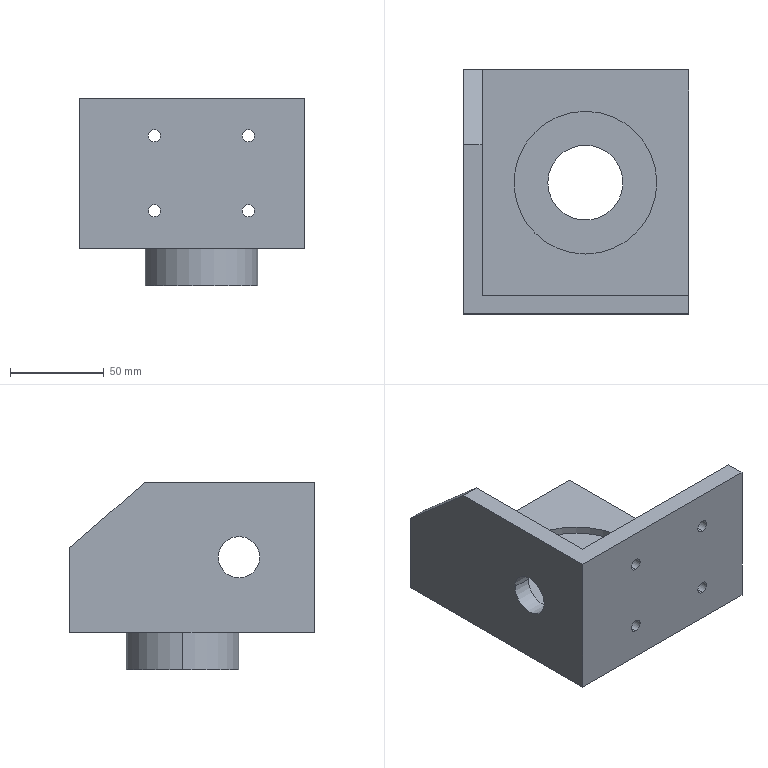Part | NX | features BREP 1 | 1 solid | 31 faces | box 120 x 130 x 100 mm | volume 300260 mm3 | cylinder 18 | plane 13 | commonest cylinder face diameters 6.5 x8 22 x2 40 x2 52 x2 60 x2 76 x2
STEP:
#1=CARTESIAN_POINT('',(-30.,0.,20.));
#2=VERTEX_POINT('',#1);
#3=CARTESIAN_POINT('',(30.,0.,20.));
#4=VERTEX_POINT('',#3);
#5=CARTESIAN_POINT('',(0.,0.,20.));
#6=DIRECTION('',(0.,0.,-1.));
#7=DIRECTION('',(-1.,0.,0.));
#8=AXIS2_PLACEMENT_3D('',#5,#6,#7);
#9=CIRCLE('',#8,30.);
#10=EDGE_CURVE('',#2,#4,#9,.T.);
#11=ORIENTED_EDGE('',*,*,#10,.T.);
#12=CARTESIAN_POINT('',(30.,0.,0.));
#13=VERTEX_POINT('',#12);
#14=CARTESIAN_POINT('',(30.,0.,20.));
#15=DIRECTION('',(0.,0.,-1.));
#16=VECTOR('',#15,1000.);
#17=LINE('',#14,#16);
#18=EDGE_CURVE('',#4,#13,#17,.T.);
#19=ORIENTED_EDGE('',*,*,#18,.T.);
#20=CARTESIAN_POINT('',(-30.,0.,0.));
#21=VERTEX_POINT('',#20);
#22=CARTESIAN_POINT('',(0.,0.,0.));
#23=DIRECTION('',(0.,0.,1.));
#24=DIRECTION('',(-1.,0.,0.));
#25=AXIS2_PLACEMENT_3D('',#22,#23,#24);
#26=CIRCLE('',#25,30.);
#27=EDGE_CURVE('',#13,#21,#26,.T.);
#28=ORIENTED_EDGE('',*,*,#27,.T.);
#29=CARTESIAN_POINT('',(-30.,0.,20.));
#30=DIRECTION('',(0.,0.,-1.));
#31=VECTOR('',#30,1000.);
#32=LINE('',#29,#31);
#33=EDGE_CURVE('',#2,#21,#32,.T.);
#34=ORIENTED_EDGE('',*,*,#33,.F.);
#35=EDGE_LOOP('',(#11,#19,#28,#34));
#36=FACE_BOUND('',#35,.T.);
#37=CARTESIAN_POINT('',(0.,0.,20.));
#38=DIRECTION('',(0.,0.,-1.));
#39=DIRECTION('',(-1.,0.,0.));
#40=AXIS2_PLACEMENT_3D('',#37,#38,#39);
#41=CYLINDRICAL_SURFACE('',#40,30.);
#42=ADVANCED_FACE('',(#36),#41,.T.);
#43=CARTESIAN_POINT('',(-25.,-60.,83.25));
#44=VERTEX_POINT('',#43);
#45=CARTESIAN_POINT('',(-25.,-60.,76.75));
#46=VERTEX_POINT('',#45);
#47=CARTESIAN_POINT('',(-25.,-60.,80.));
#48=DIRECTION('',(0.,-1.,0.));
#49=DIRECTION('',(0.,0.,-1.));
#50=AXIS2_PLACEMENT_3D('',#47,#48,#49);
#51=CIRCLE('',#50,3.25);
#52=EDGE_CURVE('',#44,#46,#51,.T.);
#53=ORIENTED_EDGE('',*,*,#52,.F.);
#54=CARTESIAN_POINT('',(-25.,-70.,83.25));
#55=VERTEX_POINT('',#54);
#56=CARTESIAN_POINT('',(-25.,-60.,83.25));
#57=DIRECTION('',(0.,-1.,0.));
#58=VECTOR('',#57,1000.);
#59=LINE('',#56,#58);
#60=EDGE_CURVE('',#44,#55,#59,.T.);
#61=ORIENTED_EDGE('',*,*,#60,.T.);
#62=CARTESIAN_POINT('',(-25.,-70.,76.75));
#63=VERTEX_POINT('',#62);
#64=CARTESIAN_POINT('',(-25.,-70.,80.));
#65=DIRECTION('',(0.,1.,0.));
#66=DIRECTION('',(0.,0.,-1.));
#67=AXIS2_PLACEMENT_3D('',#64,#65,#66);
#68=CIRCLE('',#67,3.25);
#69=EDGE_CURVE('',#63,#55,#68,.T.);
#70=ORIENTED_EDGE('',*,*,#69,.F.);
#71=CARTESIAN_POINT('',(-25.,-60.,76.75));
#72=DIRECTION('',(0.,-1.,0.));
#73=VECTOR('',#72,1000.);
#74=LINE('',#71,#73);
#75=EDGE_CURVE('',#46,#63,#74,.T.);
#76=ORIENTED_EDGE('',*,*,#75,.F.);
#77=EDGE_LOOP('',(#53,#61,#70,#76));
#78=FACE_BOUND('',#77,.T.);
#79=CARTESIAN_POINT('',(-25.,-60.,80.));
#80=DIRECTION('',(0.,-1.,0.));
#81=DIRECTION('',(0.,0.,-1.));
#82=AXIS2_PLACEMENT_3D('',#79,#80,#81);
#83=CYLINDRICAL_SURFACE('',#82,3.25);
#84=ADVANCED_FACE('',(#78),#83,.F.);
#85=CARTESIAN_POINT('',(25.,-60.,83.25));
#86=VERTEX_POINT('',#85);
#87=CARTESIAN_POINT('',(25.,-60.,76.75));
#88=VERTEX_POINT('',#87);
#89=CARTESIAN_POINT('',(25.,-60.,80.));
#90=DIRECTION('',(0.,-1.,0.));
#91=DIRECTION('',(0.,0.,-1.));
#92=AXIS2_PLACEMENT_3D('',#89,#90,#91);
#93=CIRCLE('',#92,3.25);
#94=EDGE_CURVE('',#86,#88,#93,.T.);
#95=ORIENTED_EDGE('',*,*,#94,.F.);
#96=CARTESIAN_POINT('',(25.,-70.,83.25));
#97=VERTEX_POINT('',#96);
#98=CARTESIAN_POINT('',(25.,-60.,83.25));
#99=DIRECTION('',(0.,-1.,0.));
#100=VECTOR('',#99,1000.);
#101=LINE('',#98,#100);
#102=EDGE_CURVE('',#86,#97,#101,.T.);
#103=ORIENTED_EDGE('',*,*,#102,.T.);
#104=CARTESIAN_POINT('',(25.,-70.,76.75));
#105=VERTEX_POINT('',#104);
#106=CARTESIAN_POINT('',(25.,-70.,80.));
#107=DIRECTION('',(0.,1.,0.));
#108=DIRECTION('',(0.,0.,-1.));
#109=AXIS2_PLACEMENT_3D('',#106,#107,#108);
#110=CIRCLE('',#109,3.25);
#111=EDGE_CURVE('',#105,#97,#110,.T.);
#112=ORIENTED_EDGE('',*,*,#111,.F.);
#113=CARTESIAN_POINT('',(25.,-60.,76.75));
#114=DIRECTION('',(0.,-1.,0.));
#115=VECTOR('',#114,1000.);
#116=LINE('',#113,#115);
#117=EDGE_CURVE('',#88,#105,#116,.T.);
#118=ORIENTED_EDGE('',*,*,#117,.F.);
#119=EDGE_LOOP('',(#95,#103,#112,#118));
#120=FACE_BOUND('',#119,.T.);
#121=CARTESIAN_POINT('',(25.,-60.,80.));
#122=DIRECTION('',(0.,-1.,0.));
#123=DIRECTION('',(0.,0.,-1.));
#124=AXIS2_PLACEMENT_3D('',#121,#122,#123);
#125=CYLINDRICAL_SURFACE('',#124,3.25);
#126=ADVANCED_FACE('',(#120),#125,.F.);
#127=CARTESIAN_POINT('',(25.,-60.,43.25));
#128=VERTEX_POINT('',#127);
#129=CARTESIAN_POINT('',(25.,-60.,36.75));
#130=VERTEX_POINT('',#129);
#131=CARTESIAN_POINT('',(25.,-60.,40.));
#132=DIRECTION('',(0.,-1.,0.));
#133=DIRECTION('',(0.,0.,-1.));
#134=AXIS2_PLACEMENT_3D('',#131,#132,#133);
#135=CIRCLE('',#134,3.25);
#136=EDGE_CURVE('',#128,#130,#135,.T.);
#137=ORIENTED_EDGE('',*,*,#136,.F.);
#138=CARTESIAN_POINT('',(25.,-70.,43.25));
#139=VERTEX_POINT('',#138);
#140=CARTESIAN_POINT('',(25.,-60.,43.25));
#141=DIRECTION('',(0.,-1.,0.));
#142=VECTOR('',#141,1000.);
#143=LINE('',#140,#142);
#144=EDGE_CURVE('',#128,#139,#143,.T.);
#145=ORIENTED_EDGE('',*,*,#144,.T.);
#146=CARTESIAN_POINT('',(25.,-70.,36.75));
#147=VERTEX_POINT('',#146);
#148=CARTESIAN_POINT('',(25.,-70.,40.));
#149=DIRECTION('',(0.,1.,0.));
#150=DIRECTION('',(0.,0.,-1.));
#151=AXIS2_PLACEMENT_3D('',#148,#149,#150);
#152=CIRCLE('',#151,3.25);
#153=EDGE_CURVE('',#147,#139,#152,.T.);
#154=ORIENTED_EDGE('',*,*,#153,.F.);
#155=CARTESIAN_POINT('',(25.,-60.,36.75));
#156=DIRECTION('',(0.,-1.,0.));
#157=VECTOR('',#156,1000.);
#158=LINE('',#155,#157);
#159=EDGE_CURVE('',#130,#147,#158,.T.);
#160=ORIENTED_EDGE('',*,*,#159,.F.);
#161=EDGE_LOOP('',(#137,#145,#154,#160));
#162=FACE_BOUND('',#161,.T.);
#163=CARTESIAN_POINT('',(25.,-60.,40.));
#164=DIRECTION('',(0.,-1.,0.));
#165=DIRECTION('',(0.,0.,-1.));
#166=AXIS2_PLACEMENT_3D('',#163,#164,#165);
#167=CYLINDRICAL_SURFACE('',#166,3.25);
#168=ADVANCED_FACE('',(#162),#167,.F.);
#169=CARTESIAN_POINT('',(-25.,-60.,43.25));
#170=VERTEX_POINT('',#169);
#171=CARTESIAN_POINT('',(-25.,-60.,36.75));
#172=VERTEX_POINT('',#171);
#173=CARTESIAN_POINT('',(-25.,-60.,40.));
#174=DIRECTION('',(0.,-1.,0.));
#175=DIRECTION('',(0.,0.,-1.));
#176=AXIS2_PLACEMENT_3D('',#173,#174,#175);
#177=CIRCLE('',#176,3.25);
#178=EDGE_CURVE('',#170,#172,#177,.T.);
#179=ORIENTED_EDGE('',*,*,#178,.F.);
#180=CARTESIAN_POINT('',(-25.,-70.,43.25));
#181=VERTEX_POINT('',#180);
#182=CARTESIAN_POINT('',(-25.,-60.,43.25));
#183=DIRECTION('',(0.,-1.,0.));
#184=VECTOR('',#183,1000.);
#185=LINE('',#182,#184);
#186=EDGE_CURVE('',#170,#181,#185,.T.);
#187=ORIENTED_EDGE('',*,*,#186,.T.);
#188=CARTESIAN_POINT('',(-25.,-70.,36.75));
#189=VERTEX_POINT('',#188);
#190=CARTESIAN_POINT('',(-25.,-70.,40.));
#191=DIRECTION('',(0.,1.,0.));
#192=DIRECTION('',(0.,0.,-1.));
#193=AXIS2_PLACEMENT_3D('',#190,#191,#192);
#194=CIRCLE('',#193,3.25);
#195=EDGE_CURVE('',#189,#181,#194,.T.);
#196=ORIENTED_EDGE('',*,*,#195,.F.);
#197=CARTESIAN_POINT('',(-25.,-60.,36.75));
#198=DIRECTION('',(0.,-1.,0.));
#199=VECTOR('',#198,1000.);
#200=LINE('',#197,#199);
#201=EDGE_CURVE('',#172,#189,#200,.T.);
#202=ORIENTED_EDGE('',*,*,#201,.F.);
#203=EDGE_LOOP('',(#179,#187,#196,#202));
#204=FACE_BOUND('',#203,.T.);
#205=CARTESIAN_POINT('',(-25.,-60.,40.));
#206=DIRECTION('',(0.,-1.,0.));
#207=DIRECTION('',(0.,0.,-1.));
#208=AXIS2_PLACEMENT_3D('',#205,#206,#207);
#209=CYLINDRICAL_SURFACE('',#208,3.25);
#210=ADVANCED_FACE('',(#204),#209,.F.);
#211=CARTESIAN_POINT('',(-55.,-19.,60.));
#212=VERTEX_POINT('',#211);
#213=CARTESIAN_POINT('',(-55.,-41.,60.));
#214=VERTEX_POINT('',#213);
#215=CARTESIAN_POINT('',(-55.,-30.,60.));
#216=DIRECTION('',(-1.,0.,0.));
#217=DIRECTION('',(0.,-1.,0.));
#218=AXIS2_PLACEMENT_3D('',#215,#216,#217);
#219=CIRCLE('',#218,11.);
#220=EDGE_CURVE('',#212,#214,#219,.T.);
#221=ORIENTED_EDGE('',*,*,#220,.F.);
#222=CARTESIAN_POINT('',(-65.,-19.,60.));
#223=VERTEX_POINT('',#222);
#224=CARTESIAN_POINT('',(-55.,-19.,60.));
#225=DIRECTION('',(-1.,0.,0.));
#226=VECTOR('',#225,1000.);
#227=LINE('',#224,#226);
#228=EDGE_CURVE('',#212,#223,#227,.T.);
#229=ORIENTED_EDGE('',*,*,#228,.T.);
#230=CARTESIAN_POINT('',(-65.,-41.,60.));
#231=VERTEX_POINT('',#230);
#232=CARTESIAN_POINT('',(-65.,-30.,60.));
#233=DIRECTION('',(-1.,0.,0.));
#234=DIRECTION('',(0.,-1.,0.));
#235=AXIS2_PLACEMENT_3D('',#232,#233,#234);
#236=CIRCLE('',#235,11.);
#237=EDGE_CURVE('',#223,#231,#236,.T.);
#238=ORIENTED_EDGE('',*,*,#237,.T.);
#239=CARTESIAN_POINT('',(-55.,-41.,60.));
#240=DIRECTION('',(-1.,0.,0.));
#241=VECTOR('',#240,1000.);
#242=LINE('',#239,#241);
#243=EDGE_CURVE('',#214,#231,#242,.T.);
#244=ORIENTED_EDGE('',*,*,#243,.F.);
#245=EDGE_LOOP('',(#221,#229,#238,#244));
#246=FACE_BOUND('',#245,.T.);
#247=CARTESIAN_POINT('',(-55.,-30.,60.));
#248=DIRECTION('',(-1.,0.,0.));
#249=DIRECTION('',(0.,-1.,0.));
#250=AXIS2_PLACEMENT_3D('',#247,#248,#249);
#251=CYLINDRICAL_SURFACE('',#250,11.);
#252=ADVANCED_FACE('',(#246),#251,.F.);
#253=CARTESIAN_POINT('',(26.,0.,20.));
#254=VERTEX_POINT('',#253);
#255=CARTESIAN_POINT('',(-26.,0.,20.));
#256=VERTEX_POINT('',#255);
#257=CARTESIAN_POINT('',(0.,0.,20.));
#258=DIRECTION('',(0.,0.,-1.));
#259=DIRECTION('',(-1.,0.,0.));
#260=AXIS2_PLACEMENT_3D('',#257,#258,#259);
#261=CIRCLE('',#260,26.);
#262=EDGE_CURVE('',#254,#256,#261,.T.);
#263=ORIENTED_EDGE('',*,*,#262,.F.);
#264=CARTESIAN_POINT('',(26.,0.,0.));
#265=VERTEX_POINT('',#264);
#266=CARTESIAN_POINT('',(26.,0.,20.));
#267=DIRECTION('',(0.,0.,-1.));
#268=VECTOR('',#267,1000.);
#269=LINE('',#266,#268);
#270=EDGE_CURVE('',#254,#265,#269,.T.);
#271=ORIENTED_EDGE('',*,*,#270,.T.);
#272=CARTESIAN_POINT('',(-26.,0.,0.));
#273=VERTEX_POINT('',#272);
#274=CARTESIAN_POINT('',(0.,0.,0.));
#275=DIRECTION('',(0.,0.,-1.));
#276=DIRECTION('',(-1.,0.,0.));
#277=AXIS2_PLACEMENT_3D('',#274,#275,#276);
#278=CIRCLE('',#277,26.);
#279=EDGE_CURVE('',#265,#273,#278,.T.);
#280=ORIENTED_EDGE('',*,*,#279,.T.);
#281=CARTESIAN_POINT('',(-26.,0.,20.));
#282=DIRECTION('',(0.,0.,-1.));
#283=VECTOR('',#282,1000.);
#284=LINE('',#281,#283);
#285=EDGE_CURVE('',#256,#273,#284,.T.);
#286=ORIENTED_EDGE('',*,*,#285,.F.);
#287=EDGE_LOOP('',(#263,#271,#280,#286));
#288=FACE_BOUND('',#287,.T.);
#289=CARTESIAN_POINT('',(0.,0.,20.));
#290=DIRECTION('',(0.,0.,-1.));
#291=DIRECTION('',(-1.,0.,0.));
#292=AXIS2_PLACEMENT_3D('',#289,#290,#291);
#293=CYLINDRICAL_SURFACE('',#292,26.);
#294=ADVANCED_FACE('',(#288),#293,.F.);
#295=CARTESIAN_POINT('',(-38.,0.,26.));
#296=VERTEX_POINT('',#295);
#297=CARTESIAN_POINT('',(38.,0.,26.));
#298=VERTEX_POINT('',#297);
#299=CARTESIAN_POINT('',(0.,0.,26.));
#300=DIRECTION('',(0.,0.,1.));
#301=DIRECTION('',(1.,0.,0.));
#302=AXIS2_PLACEMENT_3D('',#299,#300,#301);
#303=CIRCLE('',#302,38.);
#304=EDGE_CURVE('',#296,#298,#303,.T.);
#305=ORIENTED_EDGE('',*,*,#304,.F.);
#306=CARTESIAN_POINT('',(-38.,0.,30.));
#307=VERTEX_POINT('',#306);
#308=CARTESIAN_POINT('',(-38.,0.,26.));
#309=DIRECTION('',(0.,0.,1.));
#310=VECTOR('',#309,1000.);
#311=LINE('',#308,#310);
#312=EDGE_CURVE('',#307,#296,#311,.F.);
#313=ORIENTED_EDGE('',*,*,#312,.F.);
#314=CARTESIAN_POINT('',(38.,0.,30.));
#315=VERTEX_POINT('',#314);
#316=CARTESIAN_POINT('',(0.,0.,30.));
#317=DIRECTION('',(0.,0.,-1.));
#318=DIRECTION('',(1.,0.,0.));
#319=AXIS2_PLACEMENT_3D('',#316,#317,#318);
#320=CIRCLE('',#319,38.);
#321=EDGE_CURVE('',#315,#307,#320,.T.);
#322=ORIENTED_EDGE('',*,*,#321,.F.);
#323=CARTESIAN_POINT('',(38.,0.,26.));
#324=DIRECTION('',(0.,0.,1.));
#325=VECTOR('',#324,1000.);
#326=LINE('',#323,#325);
#327=EDGE_CURVE('',#315,#298,#326,.F.);
#328=ORIENTED_EDGE('',*,*,#327,.T.);
#329=EDGE_LOOP('',(#305,#313,#322,#328));
#330=FACE_BOUND('',#329,.T.);
#331=CARTESIAN_POINT('',(0.,0.,26.));
#332=DIRECTION('',(0.,0.,1.));
#333=DIRECTION('',(1.,0.,0.));
#334=AXIS2_PLACEMENT_3D('',#331,#332,#333);
#335=CYLINDRICAL_SURFACE('',#334,38.);
#336=ADVANCED_FACE('',(#330),#335,.F.);
#337=CARTESIAN_POINT('',(20.,0.,26.));
#338=VERTEX_POINT('',#337);
#339=CARTESIAN_POINT('',(-20.,0.,26.));
#340=VERTEX_POINT('',#339);
#341=CARTESIAN_POINT('',(0.,0.,26.));
#342=DIRECTION('',(0.,0.,-1.));
#343=DIRECTION('',(-1.,0.,0.));
#344=AXIS2_PLACEMENT_3D('',#341,#342,#343);
#345=CIRCLE('',#344,20.);
#346=EDGE_CURVE('',#338,#340,#345,.T.);
#347=ORIENTED_EDGE('',*,*,#346,.F.);
#348=CARTESIAN_POINT('',(20.,0.,20.));
#349=VERTEX_POINT('',#348);
#350=CARTESIAN_POINT('',(20.,0.,30.));
#351=DIRECTION('',(0.,0.,-1.));
#352=VECTOR('',#351,1000.);
#353=LINE('',#350,#352);
#354=EDGE_CURVE('',#338,#349,#353,.T.);
#355=ORIENTED_EDGE('',*,*,#354,.T.);
#356=CARTESIAN_POINT('',(-20.,0.,20.));
#357=VERTEX_POINT('',#356);
#358=CARTESIAN_POINT('',(0.,0.,20.));
#359=DIRECTION('',(0.,0.,-1.));
#360=DIRECTION('',(-1.,0.,0.));
#361=AXIS2_PLACEMENT_3D('',#358,#359,#360);
#362=CIRCLE('',#361,20.);
#363=EDGE_CURVE('',#349,#357,#362,.T.);
#364=ORIENTED_EDGE('',*,*,#363,.T.);
#365=CARTESIAN_POINT('',(-20.,0.,30.));
#366=DIRECTION('',(0.,0.,-1.));
#367=VECTOR('',#366,1000.);
#368=LINE('',#365,#367);
#369=EDGE_CURVE('',#340,#357,#368,.T.);
#370=ORIENTED_EDGE('',*,*,#369,.F.);
#371=EDGE_LOOP('',(#347,#355,#364,#370));
#372=FACE_BOUND('',#371,.T.);
#373=CARTESIAN_POINT('',(0.,0.,30.));
#374=DIRECTION('',(0.,0.,-1.));
#375=DIRECTION('',(-1.,0.,0.));
#376=AXIS2_PLACEMENT_3D('',#373,#374,#375);
#377=CYLINDRICAL_SURFACE('',#376,20.);
#378=ADVANCED_FACE('',(#372),#377,.F.);
#379=CARTESIAN_POINT('',(-65.,-70.,20.));
#380=VERTEX_POINT('',#379);
#381=CARTESIAN_POINT('',(55.,-70.,20.));
#382=VERTEX_POINT('',#381);
#383=CARTESIAN_POINT('',(55.,-70.,20.));
#384=DIRECTION('',(1.,0.,0.));
#385=VECTOR('',#384,1000.);
#386=LINE('',#383,#385);
#387=EDGE_CURVE('',#380,#382,#386,.T.);
#388=ORIENTED_EDGE('',*,*,#387,.F.);
#389=CARTESIAN_POINT('',(-65.,60.,20.));
#390=VERTEX_POINT('',#389);
#391=CARTESIAN_POINT('',(-65.,-60.,20.));
#392=DIRECTION('',(0.,-1.,0.));
#393=VECTOR('',#392,1000.);
#394=LINE('',#391,#393);
#395=EDGE_CURVE('',#390,#380,#394,.T.);
#396=ORIENTED_EDGE('',*,*,#395,.F.);
#397=CARTESIAN_POINT('',(55.,60.,20.));
#398=VERTEX_POINT('',#397);
#399=CARTESIAN_POINT('',(55.,60.,20.));
#400=DIRECTION('',(-1.,0.,0.));
#401=VECTOR('',#400,1000.);
#402=LINE('',#399,#401);
#403=EDGE_CURVE('',#398,#390,#402,.T.);
#404=ORIENTED_EDGE('',*,*,#403,.F.);
#405=CARTESIAN_POINT('',(55.,-60.,20.));
#406=DIRECTION('',(0.,1.,0.));
#407=VECTOR('',#406,1000.);
#408=LINE('',#405,#407);
#409=EDGE_CURVE('',#382,#398,#408,.T.);
#410=ORIENTED_EDGE('',*,*,#409,.F.);
#411=EDGE_LOOP('',(#388,#396,#404,#410));
#412=FACE_BOUND('',#411,.T.);
#413=ORIENTED_EDGE('',*,*,#10,.F.);
#414=CARTESIAN_POINT('',(0.,0.,20.));
#415=DIRECTION('',(0.,0.,-1.));
#416=DIRECTION('',(-1.,0.,0.));
#417=AXIS2_PLACEMENT_3D('',#414,#415,#416);
#418=CIRCLE('',#417,30.);
#419=EDGE_CURVE('',#4,#2,#418,.T.);
#420=ORIENTED_EDGE('',*,*,#419,.F.);
#421=EDGE_LOOP('',(#413,#420));
#422=FACE_BOUND('',#421,.T.);
#423=CARTESIAN_POINT('',(55.,-60.,20.));
#424=DIRECTION('',(0.,0.,1.));
#425=DIRECTION('',(1.,0.,0.));
#426=AXIS2_PLACEMENT_3D('',#423,#424,#425);
#427=PLANE('',#426);
#428=ADVANCED_FACE('',(#412,#422),#427,.F.);
#429=ORIENTED_EDGE('',*,*,#18,.F.);
#430=ORIENTED_EDGE('',*,*,#419,.T.);
#431=ORIENTED_EDGE('',*,*,#33,.T.);
#432=CARTESIAN_POINT('',(0.,0.,0.));
#433=DIRECTION('',(0.,0.,1.));
#434=DIRECTION('',(-1.,0.,0.));
#435=AXIS2_PLACEMENT_3D('',#432,#433,#434);
#436=CIRCLE('',#435,30.);
#437=EDGE_CURVE('',#21,#13,#436,.T.);
#438=ORIENTED_EDGE('',*,*,#437,.T.);
#439=EDGE_LOOP('',(#429,#430,#431,#438));
#440=FACE_BOUND('',#439,.T.);
#441=CARTESIAN_POINT('',(0.,0.,20.));
#442=DIRECTION('',(0.,0.,-1.));
#443=DIRECTION('',(-1.,0.,0.));
#444=AXIS2_PLACEMENT_3D('',#441,#442,#443);
#445=CYLINDRICAL_SURFACE('',#444,30.);
#446=ADVANCED_FACE('',(#440),#445,.T.);
#447=CARTESIAN_POINT('',(55.,60.,30.));
#448=VERTEX_POINT('',#447);
#449=CARTESIAN_POINT('',(55.,60.,30.));
#450=DIRECTION('',(0.,0.,-1.));
#451=VECTOR('',#450,1000.);
#452=LINE('',#449,#451);
#453=EDGE_CURVE('',#448,#398,#452,.T.);
#454=ORIENTED_EDGE('',*,*,#453,.F.);
#455=CARTESIAN_POINT('',(55.,-60.,30.));
#456=VERTEX_POINT('',#455);
#457=CARTESIAN_POINT('',(55.,60.,30.));
#458=DIRECTION('',(0.,1.,0.));
#459=VECTOR('',#458,1000.);
#460=LINE('',#457,#459);
#461=EDGE_CURVE('',#456,#448,#460,.T.);
#462=ORIENTED_EDGE('',*,*,#461,.F.);
#463=CARTESIAN_POINT('',(55.,-60.,100.));
#464=VERTEX_POINT('',#463);
#465=CARTESIAN_POINT('',(55.,-60.,30.));
#466=DIRECTION('',(0.,0.,-1.));
#467=VECTOR('',#466,1000.);
#468=LINE('',#465,#467);
#469=EDGE_CURVE('',#464,#456,#468,.T.);
#470=ORIENTED_EDGE('',*,*,#469,.F.);
#471=CARTESIAN_POINT('',(55.,-70.,100.));
#472=VERTEX_POINT('',#471);
#473=CARTESIAN_POINT('',(55.,60.,100.));
#474=DIRECTION('',(0.,1.,0.));
#475=VECTOR('',#474,1000.);
#476=LINE('',#473,#475);
#477=EDGE_CURVE('',#472,#464,#476,.T.);
#478=ORIENTED_EDGE('',*,*,#477,.F.);
#479=CARTESIAN_POINT('',(55.,-70.,30.));
#480=DIRECTION('',(0.,0.,1.));
#481=VECTOR('',#480,1000.);
#482=LINE('',#479,#481);
#483=EDGE_CURVE('',#382,#472,#482,.T.);
#484=ORIENTED_EDGE('',*,*,#483,.F.);
#485=ORIENTED_EDGE('',*,*,#409,.T.);
#486=EDGE_LOOP('',(#454,#462,#470,#478,#484,#485));
#487=FACE_BOUND('',#486,.T.);
#488=CARTESIAN_POINT('',(55.,60.,30.));
#489=DIRECTION('',(-1.,0.,0.));
#490=DIRECTION('',(0.,1.,0.));
#491=AXIS2_PLACEMENT_3D('',#488,#489,#490);
#492=PLANE('',#491);
#493=ADVANCED_FACE('',(#487),#492,.F.);
#494=ORIENTED_EDGE('',*,*,#483,.T.);
#495=CARTESIAN_POINT('',(-65.,-70.,100.));
#496=VERTEX_POINT('',#495);
#497=CARTESIAN_POINT('',(-145.623,-70.,100.));
#498=DIRECTION('',(-1.,0.,0.));
#499=VECTOR('',#498,1000.);
#500=LINE('',#497,#499);
#501=EDGE_CURVE('',#472,#496,#500,.T.);
#502=ORIENTED_EDGE('',*,*,#501,.T.);
#503=CARTESIAN_POINT('',(-65.,-70.,100.));
#504=DIRECTION('',(0.,0.,-1.));
#505=VECTOR('',#504,1000.);
#506=LINE('',#503,#505);
#507=EDGE_CURVE('',#496,#380,#506,.T.);
#508=ORIENTED_EDGE('',*,*,#507,.T.);
#509=ORIENTED_EDGE('',*,*,#387,.T.);
#510=EDGE_LOOP('',(#494,#502,#508,#509));
#511=FACE_BOUND('',#510,.T.);
#512=ORIENTED_EDGE('',*,*,#69,.T.);
#513=CARTESIAN_POINT('',(-25.,-70.,80.));
#514=DIRECTION('',(0.,1.,0.));
#515=DIRECTION('',(0.,0.,-1.));
#516=AXIS2_PLACEMENT_3D('',#513,#514,#515);
#517=CIRCLE('',#516,3.25);
#518=EDGE_CURVE('',#55,#63,#517,.T.);
#519=ORIENTED_EDGE('',*,*,#518,.T.);
#520=EDGE_LOOP('',(#512,#519));
#521=FACE_BOUND('',#520,.T.);
#522=ORIENTED_EDGE('',*,*,#111,.T.);
#523=CARTESIAN_POINT('',(25.,-70.,80.));
#524=DIRECTION('',(0.,1.,0.));
#525=DIRECTION('',(0.,0.,-1.));
#526=AXIS2_PLACEMENT_3D('',#523,#524,#525);
#527=CIRCLE('',#526,3.25);
#528=EDGE_CURVE('',#97,#105,#527,.T.);
#529=ORIENTED_EDGE('',*,*,#528,.T.);
#530=EDGE_LOOP('',(#522,#529));
#531=FACE_BOUND('',#530,.T.);
#532=ORIENTED_EDGE('',*,*,#153,.T.);
#533=CARTESIAN_POINT('',(25.,-70.,40.));
#534=DIRECTION('',(0.,1.,0.));
#535=DIRECTION('',(0.,0.,-1.));
#536=AXIS2_PLACEMENT_3D('',#533,#534,#535);
#537=CIRCLE('',#536,3.25);
#538=EDGE_CURVE('',#139,#147,#537,.T.);
#539=ORIENTED_EDGE('',*,*,#538,.T.);
#540=EDGE_LOOP('',(#532,#539));
#541=FACE_BOUND('',#540,.T.);
#542=ORIENTED_EDGE('',*,*,#195,.T.);
#543=CARTESIAN_POINT('',(-25.,-70.,40.));
#544=DIRECTION('',(0.,1.,0.));
#545=DIRECTION('',(0.,0.,-1.));
#546=AXIS2_PLACEMENT_3D('',#543,#544,#545);
#547=CIRCLE('',#546,3.25);
#548=EDGE_CURVE('',#181,#189,#547,.T.);
#549=ORIENTED_EDGE('',*,*,#548,.T.);
#550=EDGE_LOOP('',(#542,#549));
#551=FACE_BOUND('',#550,.T.);
#552=CARTESIAN_POINT('',(-145.623,-70.,100.));
#553=DIRECTION('',(0.,-1.,0.));
#554=DIRECTION('',(0.,0.,-1.));
#555=AXIS2_PLACEMENT_3D('',#552,#553,#554);
#556=PLANE('',#555);
#557=ADVANCED_FACE('',(#511,#521,#531,#541,#551),#556,.T.);
#558=ORIENTED_EDGE('',*,*,#507,.F.);
#559=CARTESIAN_POINT('',(-65.,20.,100.));
#560=VERTEX_POINT('',#559);
#561=CARTESIAN_POINT('',(-65.,60.,100.));
#562=DIRECTION('',(0.,-1.,0.));
#563=VECTOR('',#562,1000.);
#564=LINE('',#561,#563);
#565=EDGE_CURVE('',#560,#496,#564,.T.);
#566=ORIENTED_EDGE('',*,*,#565,.F.);
#567=CARTESIAN_POINT('',(-65.,60.,65.));
#568=VERTEX_POINT('',#567);
#569=CARTESIAN_POINT('',(-65.,60.,65.));
#570=DIRECTION('',(0.,-0.7526,0.6585));
#571=VECTOR('',#570,1000.);
#572=LINE('',#569,#571);
#573=EDGE_CURVE('',#568,#560,#572,.T.);
#574=ORIENTED_EDGE('',*,*,#573,.F.);
#575=CARTESIAN_POINT('',(-65.,60.,30.));
#576=DIRECTION('',(0.,0.,1.));
#577=VECTOR('',#576,1000.);
#578=LINE('',#575,#577);
#579=EDGE_CURVE('',#390,#568,#578,.T.);
#580=ORIENTED_EDGE('',*,*,#579,.F.);
#581=ORIENTED_EDGE('',*,*,#395,.T.);
#582=EDGE_LOOP('',(#558,#566,#574,#580,#581));
#583=FACE_BOUND('',#582,.T.);
#584=CARTESIAN_POINT('',(-65.,-30.,60.));
#585=DIRECTION('',(-1.,0.,0.));
#586=DIRECTION('',(0.,-1.,0.));
#587=AXIS2_PLACEMENT_3D('',#584,#585,#586);
#588=CIRCLE('',#587,11.);
#589=EDGE_CURVE('',#231,#223,#588,.T.);
#590=ORIENTED_EDGE('',*,*,#589,.F.);
#591=ORIENTED_EDGE('',*,*,#237,.F.);
#592=EDGE_LOOP('',(#590,#591));
#593=FACE_BOUND('',#592,.T.);
#594=CARTESIAN_POINT('',(-65.,60.,30.));
#595=DIRECTION('',(1.,0.,0.));
#596=DIRECTION('',(0.,1.,0.));
#597=AXIS2_PLACEMENT_3D('',#594,#595,#596);
#598=PLANE('',#597);
#599=ADVANCED_FACE('',(#583,#593),#598,.F.);
#600=ORIENTED_EDGE('',*,*,#579,.T.);
#601=CARTESIAN_POINT('',(-55.,60.,65.));
#602=VERTEX_POINT('',#601);
#603=CARTESIAN_POINT('',(-65.,60.,65.));
#604=DIRECTION('',(-1.,0.,0.));
#605=VECTOR('',#604,1000.);
#606=LINE('',#603,#605);
#607=EDGE_CURVE('',#602,#568,#606,.T.);
#608=ORIENTED_EDGE('',*,*,#607,.F.);
#609=CARTESIAN_POINT('',(-55.,60.,30.));
#610=VERTEX_POINT('',#609);
#611=CARTESIAN_POINT('',(-55.,60.,30.));
#612=DIRECTION('',(0.,0.,1.));
#613=VECTOR('',#612,1000.);
#614=LINE('',#611,#613);
#615=EDGE_CURVE('',#610,#602,#614,.T.);
#616=ORIENTED_EDGE('',*,*,#615,.F.);
#617=CARTESIAN_POINT('',(-65.,60.,30.));
#618=DIRECTION('',(-1.,0.,0.));
#619=VECTOR('',#618,1000.);
#620=LINE('',#617,#619);
#621=EDGE_CURVE('',#448,#610,#620,.T.);
#622=ORIENTED_EDGE('',*,*,#621,.F.);
#623=ORIENTED_EDGE('',*,*,#453,.T.);
#624=ORIENTED_EDGE('',*,*,#403,.T.);
#625=EDGE_LOOP('',(#600,#608,#616,#622,#623,#624));
#626=FACE_BOUND('',#625,.T.);
#627=CARTESIAN_POINT('',(-65.,60.,30.));
#628=DIRECTION('',(0.,-1.,0.));
#629=DIRECTION('',(0.,0.,-1.));
#630=AXIS2_PLACEMENT_3D('',#627,#628,#629);
#631=PLANE('',#630);
#632=ADVANCED_FACE('',(#626),#631,.F.);
#633=ORIENTED_EDGE('',*,*,#437,.F.);
#634=ORIENTED_EDGE('',*,*,#27,.F.);
#635=EDGE_LOOP('',(#633,#634));
#636=FACE_BOUND('',#635,.T.);
#637=CARTESIAN_POINT('',(0.,0.,0.));
#638=DIRECTION('',(0.,0.,-1.));
#639=DIRECTION('',(-1.,0.,0.));
#640=AXIS2_PLACEMENT_3D('',#637,#638,#639);
#641=CIRCLE('',#640,26.);
#642=EDGE_CURVE('',#273,#265,#641,.T.);
#643=ORIENTED_EDGE('',*,*,#642,.F.);
#644=ORIENTED_EDGE('',*,*,#279,.F.);
#645=EDGE_LOOP('',(#643,#644));
#646=FACE_BOUND('',#645,.T.);
#647=CARTESIAN_POINT('',(0.,0.,0.));
#648=DIRECTION('',(0.,0.,1.));
#649=DIRECTION('',(1.,0.,0.));
#650=AXIS2_PLACEMENT_3D('',#647,#648,#649);
#651=PLANE('',#650);
#652=ADVANCED_FACE('',(#636,#646),#651,.F.);
#653=CARTESIAN_POINT('',(-55.,-60.,30.));
#654=VERTEX_POINT('',#653);
#655=CARTESIAN_POINT('',(55.,-60.,30.));
#656=DIRECTION('',(1.,0.,0.));
#657=VECTOR('',#656,1000.);
#658=LINE('',#655,#657);
#659=EDGE_CURVE('',#654,#456,#658,.T.);
#660=ORIENTED_EDGE('',*,*,#659,.T.);
#661=ORIENTED_EDGE('',*,*,#461,.T.);
#662=ORIENTED_EDGE('',*,*,#621,.T.);
#663=CARTESIAN_POINT('',(-55.,-60.,30.));
#664=DIRECTION('',(0.,-1.,0.));
#665=VECTOR('',#664,1000.);
#666=LINE('',#663,#665);
#667=EDGE_CURVE('',#610,#654,#666,.T.);
#668=ORIENTED_EDGE('',*,*,#667,.T.);
#669=EDGE_LOOP('',(#660,#661,#662,#668));
#670=FACE_BOUND('',#669,.T.);
#671=ORIENTED_EDGE('',*,*,#321,.T.);
#672=CARTESIAN_POINT('',(0.,0.,30.));
#673=DIRECTION('',(0.,0.,-1.));
#674=DIRECTION('',(1.,0.,0.));
#675=AXIS2_PLACEMENT_3D('',#672,#673,#674);
#676=CIRCLE('',#675,38.);
#677=EDGE_CURVE('',#307,#315,#676,.T.);
#678=ORIENTED_EDGE('',*,*,#677,.T.);
#679=EDGE_LOOP('',(#671,#678));
#680=FACE_BOUND('',#679,.T.);
#681=CARTESIAN_POINT('',(55.,-60.,30.));
#682=DIRECTION('',(0.,0.,1.));
#683=DIRECTION('',(1.,0.,0.));
#684=AXIS2_PLACEMENT_3D('',#681,#682,#683);
#685=PLANE('',#684);
#686=ADVANCED_FACE('',(#670,#680),#685,.T.);
#687=CARTESIAN_POINT('',(-55.,-60.,100.));
#688=VERTEX_POINT('',#687);
#689=CARTESIAN_POINT('',(-145.623,-60.,100.));
#690=DIRECTION('',(1.,0.,0.));
#691=VECTOR('',#690,1000.);
#692=LINE('',#689,#691);
#693=EDGE_CURVE('',#688,#464,#692,.T.);
#694=ORIENTED_EDGE('',*,*,#693,.T.);
#695=ORIENTED_EDGE('',*,*,#469,.T.);
#696=ORIENTED_EDGE('',*,*,#659,.F.);
#697=CARTESIAN_POINT('',(-55.,-60.,100.));
#698=DIRECTION('',(0.,0.,1.));
#699=VECTOR('',#698,1000.);
#700=LINE('',#697,#699);
#701=EDGE_CURVE('',#654,#688,#700,.T.);
#702=ORIENTED_EDGE('',*,*,#701,.T.);
#703=EDGE_LOOP('',(#694,#695,#696,#702));
#704=FACE_BOUND('',#703,.T.);
#705=CARTESIAN_POINT('',(-25.,-60.,80.));
#706=DIRECTION('',(0.,-1.,0.));
#707=DIRECTION('',(0.,0.,-1.));
#708=AXIS2_PLACEMENT_3D('',#705,#706,#707);
#709=CIRCLE('',#708,3.25);
#710=EDGE_CURVE('',#46,#44,#709,.T.);
#711=ORIENTED_EDGE('',*,*,#710,.T.);
#712=ORIENTED_EDGE('',*,*,#52,.T.);
#713=EDGE_LOOP('',(#711,#712));
#714=FACE_BOUND('',#713,.T.);
#715=CARTESIAN_POINT('',(25.,-60.,80.));
#716=DIRECTION('',(0.,-1.,0.));
#717=DIRECTION('',(0.,0.,-1.));
#718=AXIS2_PLACEMENT_3D('',#715,#716,#717);
#719=CIRCLE('',#718,3.25);
#720=EDGE_CURVE('',#88,#86,#719,.T.);
#721=ORIENTED_EDGE('',*,*,#720,.T.);
#722=ORIENTED_EDGE('',*,*,#94,.T.);
#723=EDGE_LOOP('',(#721,#722));
#724=FACE_BOUND('',#723,.T.);
#725=CARTESIAN_POINT('',(25.,-60.,40.));
#726=DIRECTION('',(0.,-1.,0.));
#727=DIRECTION('',(0.,0.,-1.));
#728=AXIS2_PLACEMENT_3D('',#725,#726,#727);
#729=CIRCLE('',#728,3.25);
#730=EDGE_CURVE('',#130,#128,#729,.T.);
#731=ORIENTED_EDGE('',*,*,#730,.T.);
#732=ORIENTED_EDGE('',*,*,#136,.T.);
#733=EDGE_LOOP('',(#731,#732));
#734=FACE_BOUND('',#733,.T.);
#735=CARTESIAN_POINT('',(-25.,-60.,40.));
#736=DIRECTION('',(0.,-1.,0.));
#737=DIRECTION('',(0.,0.,-1.));
#738=AXIS2_PLACEMENT_3D('',#735,#736,#737);
#739=CIRCLE('',#738,3.25);
#740=EDGE_CURVE('',#172,#170,#739,.T.);
#741=ORIENTED_EDGE('',*,*,#740,.T.);
#742=ORIENTED_EDGE('',*,*,#178,.T.);
#743=EDGE_LOOP('',(#741,#742));
#744=FACE_BOUND('',#743,.T.);
#745=CARTESIAN_POINT('',(-145.623,-60.,100.));
#746=DIRECTION('',(0.,1.,0.));
#747=DIRECTION('',(1.,0.,0.));
#748=AXIS2_PLACEMENT_3D('',#745,#746,#747);
#749=PLANE('',#748);
#750=ADVANCED_FACE('',(#704,#714,#724,#734,#744),#749,.T.);
#751=CARTESIAN_POINT('',(-55.,20.,100.));
#752=VERTEX_POINT('',#751);
#753=CARTESIAN_POINT('',(-55.,-60.,100.));
#754=DIRECTION('',(0.,1.,0.));
#755=VECTOR('',#754,1000.);
#756=LINE('',#753,#755);
#757=EDGE_CURVE('',#688,#752,#756,.T.);
#758=ORIENTED_EDGE('',*,*,#757,.T.);
#759=CARTESIAN_POINT('',(-145.623,20.,100.));
#760=DIRECTION('',(-1.,0.,0.));
#761=VECTOR('',#760,1000.);
#762=LINE('',#759,#761);
#763=EDGE_CURVE('',#752,#560,#762,.T.);
#764=ORIENTED_EDGE('',*,*,#763,.T.);
#765=ORIENTED_EDGE('',*,*,#565,.T.);
#766=ORIENTED_EDGE('',*,*,#501,.F.);
#767=ORIENTED_EDGE('',*,*,#477,.T.);
#768=ORIENTED_EDGE('',*,*,#693,.F.);
#769=EDGE_LOOP('',(#758,#764,#765,#766,#767,#768));
#770=FACE_BOUND('',#769,.T.);
#771=CARTESIAN_POINT('',(-145.623,-60.,100.));
#772=DIRECTION('',(0.,0.,1.));
#773=DIRECTION('',(1.,0.,0.));
#774=AXIS2_PLACEMENT_3D('',#771,#772,#773);
#775=PLANE('',#774);
#776=ADVANCED_FACE('',(#770),#775,.T.);
#777=ORIENTED_EDGE('',*,*,#60,.F.);
#778=ORIENTED_EDGE('',*,*,#710,.F.);
#779=ORIENTED_EDGE('',*,*,#75,.T.);
#780=ORIENTED_EDGE('',*,*,#518,.F.);
#781=EDGE_LOOP('',(#777,#778,#779,#780));
#782=FACE_BOUND('',#781,.T.);
#783=CARTESIAN_POINT('',(-25.,-60.,80.));
#784=DIRECTION('',(0.,-1.,0.));
#785=DIRECTION('',(0.,0.,-1.));
#786=AXIS2_PLACEMENT_3D('',#783,#784,#785);
#787=CYLINDRICAL_SURFACE('',#786,3.25);
#788=ADVANCED_FACE('',(#782),#787,.F.);
#789=ORIENTED_EDGE('',*,*,#102,.F.);
#790=ORIENTED_EDGE('',*,*,#720,.F.);
#791=ORIENTED_EDGE('',*,*,#117,.T.);
#792=ORIENTED_EDGE('',*,*,#528,.F.);
#793=EDGE_LOOP('',(#789,#790,#791,#792));
#794=FACE_BOUND('',#793,.T.);
#795=CARTESIAN_POINT('',(25.,-60.,80.));
#796=DIRECTION('',(0.,-1.,0.));
#797=DIRECTION('',(0.,0.,-1.));
#798=AXIS2_PLACEMENT_3D('',#795,#796,#797);
#799=CYLINDRICAL_SURFACE('',#798,3.25);
#800=ADVANCED_FACE('',(#794),#799,.F.);
#801=ORIENTED_EDGE('',*,*,#144,.F.);
#802=ORIENTED_EDGE('',*,*,#730,.F.);
#803=ORIENTED_EDGE('',*,*,#159,.T.);
#804=ORIENTED_EDGE('',*,*,#538,.F.);
#805=EDGE_LOOP('',(#801,#802,#803,#804));
#806=FACE_BOUND('',#805,.T.);
#807=CARTESIAN_POINT('',(25.,-60.,40.));
#808=DIRECTION('',(0.,-1.,0.));
#809=DIRECTION('',(0.,0.,-1.));
#810=AXIS2_PLACEMENT_3D('',#807,#808,#809);
#811=CYLINDRICAL_SURFACE('',#810,3.25);
#812=ADVANCED_FACE('',(#806),#811,.F.);
#813=ORIENTED_EDGE('',*,*,#186,.F.);
#814=ORIENTED_EDGE('',*,*,#740,.F.);
#815=ORIENTED_EDGE('',*,*,#201,.T.);
#816=ORIENTED_EDGE('',*,*,#548,.F.);
#817=EDGE_LOOP('',(#813,#814,#815,#816));
#818=FACE_BOUND('',#817,.T.);
#819=CARTESIAN_POINT('',(-25.,-60.,40.));
#820=DIRECTION('',(0.,-1.,0.));
#821=DIRECTION('',(0.,0.,-1.));
#822=AXIS2_PLACEMENT_3D('',#819,#820,#821);
#823=CYLINDRICAL_SURFACE('',#822,3.25);
#824=ADVANCED_FACE('',(#818),#823,.F.);
#825=CARTESIAN_POINT('',(-55.,20.,100.));
#826=DIRECTION('',(0.,0.7526,-0.6585));
#827=VECTOR('',#826,1000.);
#828=LINE('',#825,#827);
#829=EDGE_CURVE('',#752,#602,#828,.T.);
#830=ORIENTED_EDGE('',*,*,#829,.T.);
#831=ORIENTED_EDGE('',*,*,#607,.T.);
#832=ORIENTED_EDGE('',*,*,#573,.T.);
#833=ORIENTED_EDGE('',*,*,#763,.F.);
#834=EDGE_LOOP('',(#830,#831,#832,#833));
#835=FACE_BOUND('',#834,.T.);
#836=CARTESIAN_POINT('',(-55.,20.,100.));
#837=DIRECTION('',(0.,0.6585,0.7526));
#838=DIRECTION('',(1.,0.,0.));
#839=AXIS2_PLACEMENT_3D('',#836,#837,#838);
#840=PLANE('',#839);
#841=ADVANCED_FACE('',(#835),#840,.T.);
#842=ORIENTED_EDGE('',*,*,#228,.F.);
#843=CARTESIAN_POINT('',(-55.,-30.,60.));
#844=DIRECTION('',(-1.,0.,0.));
#845=DIRECTION('',(0.,-1.,0.));
#846=AXIS2_PLACEMENT_3D('',#843,#844,#845);
#847=CIRCLE('',#846,11.);
#848=EDGE_CURVE('',#214,#212,#847,.T.);
#849=ORIENTED_EDGE('',*,*,#848,.F.);
#850=ORIENTED_EDGE('',*,*,#243,.T.);
#851=ORIENTED_EDGE('',*,*,#589,.T.);
#852=EDGE_LOOP('',(#842,#849,#850,#851));
#853=FACE_BOUND('',#852,.T.);
#854=CARTESIAN_POINT('',(-55.,-30.,60.));
#855=DIRECTION('',(-1.,0.,0.));
#856=DIRECTION('',(0.,-1.,0.));
#857=AXIS2_PLACEMENT_3D('',#854,#855,#856);
#858=CYLINDRICAL_SURFACE('',#857,11.);
#859=ADVANCED_FACE('',(#853),#858,.F.);
#860=ORIENTED_EDGE('',*,*,#829,.F.);
#861=ORIENTED_EDGE('',*,*,#757,.F.);
#862=ORIENTED_EDGE('',*,*,#701,.F.);
#863=ORIENTED_EDGE('',*,*,#667,.F.);
#864=ORIENTED_EDGE('',*,*,#615,.T.);
#865=EDGE_LOOP('',(#860,#861,#862,#863,#864));
#866=FACE_BOUND('',#865,.T.);
#867=ORIENTED_EDGE('',*,*,#848,.T.);
#868=ORIENTED_EDGE('',*,*,#220,.T.);
#869=EDGE_LOOP('',(#867,#868));
#870=FACE_BOUND('',#869,.T.);
#871=CARTESIAN_POINT('',(-55.,60.,30.));
#872=DIRECTION('',(-1.,0.,0.));
#873=DIRECTION('',(0.,0.,1.));
#874=AXIS2_PLACEMENT_3D('',#871,#872,#873);
#875=PLANE('',#874);
#876=ADVANCED_FACE('',(#866,#870),#875,.F.);
#877=ORIENTED_EDGE('',*,*,#270,.F.);
#878=CARTESIAN_POINT('',(0.,0.,20.));
#879=DIRECTION('',(0.,0.,-1.));
#880=DIRECTION('',(-1.,0.,0.));
#881=AXIS2_PLACEMENT_3D('',#878,#879,#880);
#882=CIRCLE('',#881,26.);
#883=EDGE_CURVE('',#256,#254,#882,.T.);
#884=ORIENTED_EDGE('',*,*,#883,.F.);
#885=ORIENTED_EDGE('',*,*,#285,.T.);
#886=ORIENTED_EDGE('',*,*,#642,.T.);
#887=EDGE_LOOP('',(#877,#884,#885,#886));
#888=FACE_BOUND('',#887,.T.);
#889=CARTESIAN_POINT('',(0.,0.,20.));
#890=DIRECTION('',(0.,0.,-1.));
#891=DIRECTION('',(-1.,0.,0.));
#892=AXIS2_PLACEMENT_3D('',#889,#890,#891);
#893=CYLINDRICAL_SURFACE('',#892,26.);
#894=ADVANCED_FACE('',(#888),#893,.F.);
#895=ORIENTED_EDGE('',*,*,#312,.T.);
#896=CARTESIAN_POINT('',(0.,0.,26.));
#897=DIRECTION('',(0.,0.,1.));
#898=DIRECTION('',(1.,0.,0.));
#899=AXIS2_PLACEMENT_3D('',#896,#897,#898);
#900=CIRCLE('',#899,38.);
#901=EDGE_CURVE('',#298,#296,#900,.T.);
#902=ORIENTED_EDGE('',*,*,#901,.F.);
#903=ORIENTED_EDGE('',*,*,#327,.F.);
#904=ORIENTED_EDGE('',*,*,#677,.F.);
#905=EDGE_LOOP('',(#895,#902,#903,#904));
#906=FACE_BOUND('',#905,.T.);
#907=CARTESIAN_POINT('',(0.,0.,26.));
#908=DIRECTION('',(0.,0.,1.));
#909=DIRECTION('',(1.,0.,0.));
#910=AXIS2_PLACEMENT_3D('',#907,#908,#909);
#911=CYLINDRICAL_SURFACE('',#910,38.);
#912=ADVANCED_FACE('',(#906),#911,.F.);
#913=ORIENTED_EDGE('',*,*,#883,.T.);
#914=ORIENTED_EDGE('',*,*,#262,.T.);
#915=EDGE_LOOP('',(#913,#914));
#916=FACE_BOUND('',#915,.T.);
#917=CARTESIAN_POINT('',(0.,0.,20.));
#918=DIRECTION('',(0.,0.,-1.));
#919=DIRECTION('',(-1.,0.,0.));
#920=AXIS2_PLACEMENT_3D('',#917,#918,#919);
#921=CIRCLE('',#920,20.);
#922=EDGE_CURVE('',#357,#349,#921,.T.);
#923=ORIENTED_EDGE('',*,*,#922,.F.);
#924=ORIENTED_EDGE('',*,*,#363,.F.);
#925=EDGE_LOOP('',(#923,#924));
#926=FACE_BOUND('',#925,.T.);
#927=CARTESIAN_POINT('',(55.,-60.,20.));
#928=DIRECTION('',(0.,0.,1.));
#929=DIRECTION('',(1.,0.,0.));
#930=AXIS2_PLACEMENT_3D('',#927,#928,#929);
#931=PLANE('',#930);
#932=ADVANCED_FACE('',(#916,#926),#931,.F.);
#933=ORIENTED_EDGE('',*,*,#901,.T.);
#934=ORIENTED_EDGE('',*,*,#304,.T.);
#935=EDGE_LOOP('',(#933,#934));
#936=FACE_BOUND('',#935,.T.);
#937=CARTESIAN_POINT('',(0.,0.,26.));
#938=DIRECTION('',(0.,0.,-1.));
#939=DIRECTION('',(-1.,0.,0.));
#940=AXIS2_PLACEMENT_3D('',#937,#938,#939);
#941=CIRCLE('',#940,20.);
#942=EDGE_CURVE('',#340,#338,#941,.T.);
#943=ORIENTED_EDGE('',*,*,#942,.T.);
#944=ORIENTED_EDGE('',*,*,#346,.T.);
#945=EDGE_LOOP('',(#943,#944));
#946=FACE_BOUND('',#945,.T.);
#947=CARTESIAN_POINT('',(0.,0.,26.));
#948=DIRECTION('',(0.,0.,1.));
#949=DIRECTION('',(1.,0.,0.));
#950=AXIS2_PLACEMENT_3D('',#947,#948,#949);
#951=PLANE('',#950);
#952=ADVANCED_FACE('',(#936,#946),#951,.T.);
#953=ORIENTED_EDGE('',*,*,#354,.F.);
#954=ORIENTED_EDGE('',*,*,#942,.F.);
#955=ORIENTED_EDGE('',*,*,#369,.T.);
#956=ORIENTED_EDGE('',*,*,#922,.T.);
#957=EDGE_LOOP('',(#953,#954,#955,#956));
#958=FACE_BOUND('',#957,.T.);
#959=CARTESIAN_POINT('',(0.,0.,30.));
#960=DIRECTION('',(0.,0.,-1.));
#961=DIRECTION('',(-1.,0.,0.));
#962=AXIS2_PLACEMENT_3D('',#959,#960,#961);
#963=CYLINDRICAL_SURFACE('',#962,20.);
#964=ADVANCED_FACE('',(#958),#963,.F.);
#965=CLOSED_SHELL('',(#42,#84,#126,#168,#210,#252,#294,#336,#378,#428,#446,#493,#557,#599,#632,#652,#686,#750,#776,#788,#800,#812,#824,#841,#859,#876,#894,#912,#932,#952,#964));
#966=MANIFOLD_SOLID_BREP('',#965);
#967=(LENGTH_UNIT()NAMED_UNIT(*)SI_UNIT(.MILLI.,.METRE.));
#968=UNCERTAINTY_MEASURE_WITH_UNIT(LENGTH_MEASURE(0.00001),#967,'','');
#969=(NAMED_UNIT(*)PLANE_ANGLE_UNIT()SI_UNIT($,.RADIAN.));
#970=(NAMED_UNIT(*)SI_UNIT($,.STERADIAN.)SOLID_ANGLE_UNIT());
#971=(GEOMETRIC_REPRESENTATION_CONTEXT(3)GLOBAL_UNCERTAINTY_ASSIGNED_CONTEXT((#968))GLOBAL_UNIT_ASSIGNED_CONTEXT((#967,#969,#970))REPRESENTATION_CONTEXT('',''));
#972=ADVANCED_BREP_SHAPE_REPRESENTATION('',(#966),#971);